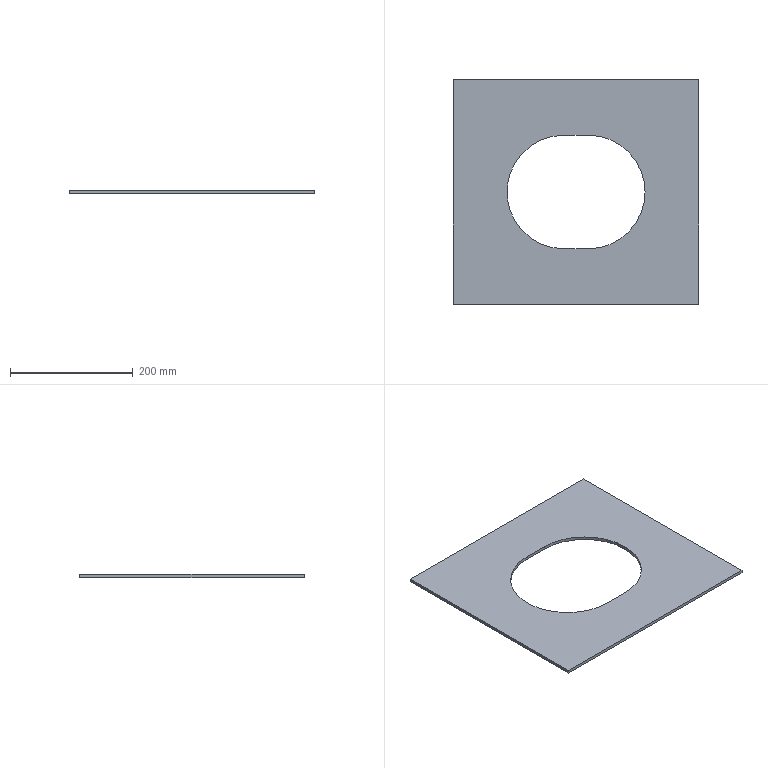Part | SolidWorks | features Extrusion 1, ICE 1 | 1 solid | 11 faces | box 400 x 365 x 5 mm | volume 558599 mm3 | plane 8 | cylinder 3 | commonest cylinder face diameters 185 x3
STEP:
#1=CARTESIAN_POINT('',(312.5,182.5,0.));
#2=VERTEX_POINT('',#1);
#3=CARTESIAN_POINT('',(220.,275.,0.));
#4=VERTEX_POINT('',#3);
#5=CARTESIAN_POINT('',(220.,182.5,0.));
#6=DIRECTION('',(0.,0.,1.));
#7=DIRECTION('',(1.,0.,0.));
#8=AXIS2_PLACEMENT_3D('',#5,#6,#7);
#9=CIRCLE('',#8,92.5);
#10=EDGE_CURVE('',#2,#4,#9,.T.);
#11=ORIENTED_EDGE('',*,*,#10,.F.);
#12=CARTESIAN_POINT('',(312.5,182.5,5.));
#13=VERTEX_POINT('',#12);
#14=CARTESIAN_POINT('',(312.5,182.5,-5.));
#15=DIRECTION('',(0.,0.,1.));
#16=VECTOR('',#15,1000.);
#17=LINE('',#14,#16);
#18=EDGE_CURVE('',#2,#13,#17,.T.);
#19=ORIENTED_EDGE('',*,*,#18,.T.);
#20=CARTESIAN_POINT('',(220.,275.,5.));
#21=VERTEX_POINT('',#20);
#22=CARTESIAN_POINT('',(220.,182.5,5.));
#23=DIRECTION('',(0.,0.,1.));
#24=DIRECTION('',(1.,0.,0.));
#25=AXIS2_PLACEMENT_3D('',#22,#23,#24);
#26=CIRCLE('',#25,92.5);
#27=EDGE_CURVE('',#13,#21,#26,.T.);
#28=ORIENTED_EDGE('',*,*,#27,.T.);
#29=CARTESIAN_POINT('',(220.,275.,-5.));
#30=DIRECTION('',(0.,0.,1.));
#31=VECTOR('',#30,1000.);
#32=LINE('',#29,#31);
#33=EDGE_CURVE('',#4,#21,#32,.T.);
#34=ORIENTED_EDGE('',*,*,#33,.F.);
#35=EDGE_LOOP('',(#11,#19,#28,#34));
#36=FACE_OUTER_BOUND('',#35,.T.);
#37=CARTESIAN_POINT('',(220.,182.5,-5.));
#38=DIRECTION('',(0.,0.,1.));
#39=DIRECTION('',(1.,0.,0.));
#40=AXIS2_PLACEMENT_3D('',#37,#38,#39);
#41=CYLINDRICAL_SURFACE('',#40,92.5);
#42=ADVANCED_FACE('',(#36),#41,.F.);
#43=CARTESIAN_POINT('',(0.,365.,0.));
#44=VERTEX_POINT('',#43);
#45=CARTESIAN_POINT('',(0.,0.,0.));
#46=VERTEX_POINT('',#45);
#47=CARTESIAN_POINT('',(0.,365.,0.));
#48=DIRECTION('',(0.,-1.,0.));
#49=VECTOR('',#48,1000.);
#50=LINE('',#47,#49);
#51=EDGE_CURVE('',#44,#46,#50,.T.);
#52=ORIENTED_EDGE('',*,*,#51,.T.);
#53=CARTESIAN_POINT('',(0.,0.,5.));
#54=VERTEX_POINT('',#53);
#55=CARTESIAN_POINT('',(0.,0.,5.));
#56=DIRECTION('',(0.,0.,-1.));
#57=VECTOR('',#56,1000.);
#58=LINE('',#55,#57);
#59=EDGE_CURVE('',#54,#46,#58,.T.);
#60=ORIENTED_EDGE('',*,*,#59,.F.);
#61=CARTESIAN_POINT('',(0.,365.,5.));
#62=VERTEX_POINT('',#61);
#63=CARTESIAN_POINT('',(0.,365.,5.));
#64=DIRECTION('',(0.,-1.,0.));
#65=VECTOR('',#64,1000.);
#66=LINE('',#63,#65);
#67=EDGE_CURVE('',#62,#54,#66,.T.);
#68=ORIENTED_EDGE('',*,*,#67,.F.);
#69=CARTESIAN_POINT('',(0.,365.,5.));
#70=DIRECTION('',(0.,0.,-1.));
#71=VECTOR('',#70,1000.);
#72=LINE('',#69,#71);
#73=EDGE_CURVE('',#62,#44,#72,.T.);
#74=ORIENTED_EDGE('',*,*,#73,.T.);
#75=EDGE_LOOP('',(#52,#60,#68,#74));
#76=FACE_OUTER_BOUND('',#75,.T.);
#77=CARTESIAN_POINT('',(0.,365.,5.));
#78=DIRECTION('',(1.,0.,0.));
#79=DIRECTION('',(0.,0.,-1.));
#80=AXIS2_PLACEMENT_3D('',#77,#78,#79);
#81=PLANE('',#80);
#82=ADVANCED_FACE('',(#76),#81,.F.);
#83=CARTESIAN_POINT('',(400.,0.,0.));
#84=VERTEX_POINT('',#83);
#85=CARTESIAN_POINT('',(0.,0.,0.));
#86=DIRECTION('',(1.,0.,0.));
#87=VECTOR('',#86,1000.);
#88=LINE('',#85,#87);
#89=EDGE_CURVE('',#46,#84,#88,.T.);
#90=ORIENTED_EDGE('',*,*,#89,.T.);
#91=CARTESIAN_POINT('',(400.,0.,5.));
#92=VERTEX_POINT('',#91);
#93=CARTESIAN_POINT('',(400.,0.,5.));
#94=DIRECTION('',(0.,0.,-1.));
#95=VECTOR('',#94,1000.);
#96=LINE('',#93,#95);
#97=EDGE_CURVE('',#92,#84,#96,.T.);
#98=ORIENTED_EDGE('',*,*,#97,.F.);
#99=CARTESIAN_POINT('',(0.,0.,5.));
#100=DIRECTION('',(1.,0.,0.));
#101=VECTOR('',#100,1000.);
#102=LINE('',#99,#101);
#103=EDGE_CURVE('',#54,#92,#102,.T.);
#104=ORIENTED_EDGE('',*,*,#103,.F.);
#105=ORIENTED_EDGE('',*,*,#59,.T.);
#106=EDGE_LOOP('',(#90,#98,#104,#105));
#107=FACE_OUTER_BOUND('',#106,.T.);
#108=CARTESIAN_POINT('',(0.,0.,5.));
#109=DIRECTION('',(0.,1.,0.));
#110=DIRECTION('',(0.,0.,1.));
#111=AXIS2_PLACEMENT_3D('',#108,#109,#110);
#112=PLANE('',#111);
#113=ADVANCED_FACE('',(#107),#112,.F.);
#114=CARTESIAN_POINT('',(400.,365.,0.));
#115=VERTEX_POINT('',#114);
#116=CARTESIAN_POINT('',(400.,0.,0.));
#117=DIRECTION('',(0.,1.,0.));
#118=VECTOR('',#117,1000.);
#119=LINE('',#116,#118);
#120=EDGE_CURVE('',#84,#115,#119,.T.);
#121=ORIENTED_EDGE('',*,*,#120,.T.);
#122=CARTESIAN_POINT('',(400.,365.,5.));
#123=VERTEX_POINT('',#122);
#124=CARTESIAN_POINT('',(400.,365.,5.));
#125=DIRECTION('',(0.,0.,-1.));
#126=VECTOR('',#125,1000.);
#127=LINE('',#124,#126);
#128=EDGE_CURVE('',#123,#115,#127,.T.);
#129=ORIENTED_EDGE('',*,*,#128,.F.);
#130=CARTESIAN_POINT('',(400.,0.,5.));
#131=DIRECTION('',(0.,1.,0.));
#132=VECTOR('',#131,1000.);
#133=LINE('',#130,#132);
#134=EDGE_CURVE('',#92,#123,#133,.T.);
#135=ORIENTED_EDGE('',*,*,#134,.F.);
#136=ORIENTED_EDGE('',*,*,#97,.T.);
#137=EDGE_LOOP('',(#121,#129,#135,#136));
#138=FACE_OUTER_BOUND('',#137,.T.);
#139=CARTESIAN_POINT('',(400.,0.,5.));
#140=DIRECTION('',(-1.,0.,0.));
#141=DIRECTION('',(0.,0.,1.));
#142=AXIS2_PLACEMENT_3D('',#139,#140,#141);
#143=PLANE('',#142);
#144=ADVANCED_FACE('',(#138),#143,.F.);
#145=CARTESIAN_POINT('',(400.,365.,0.));
#146=DIRECTION('',(-1.,0.,0.));
#147=VECTOR('',#146,1000.);
#148=LINE('',#145,#147);
#149=EDGE_CURVE('',#115,#44,#148,.T.);
#150=ORIENTED_EDGE('',*,*,#149,.T.);
#151=ORIENTED_EDGE('',*,*,#73,.F.);
#152=CARTESIAN_POINT('',(400.,365.,5.));
#153=DIRECTION('',(-1.,0.,0.));
#154=VECTOR('',#153,1000.);
#155=LINE('',#152,#154);
#156=EDGE_CURVE('',#123,#62,#155,.T.);
#157=ORIENTED_EDGE('',*,*,#156,.F.);
#158=ORIENTED_EDGE('',*,*,#128,.T.);
#159=EDGE_LOOP('',(#150,#151,#157,#158));
#160=FACE_OUTER_BOUND('',#159,.T.);
#161=CARTESIAN_POINT('',(400.,365.,5.));
#162=DIRECTION('',(0.,-1.,0.));
#163=DIRECTION('',(0.,0.,-1.));
#164=AXIS2_PLACEMENT_3D('',#161,#162,#163);
#165=PLANE('',#164);
#166=ADVANCED_FACE('',(#160),#165,.F.);
#167=CARTESIAN_POINT('',(180.,275.,5.));
#168=VERTEX_POINT('',#167);
#169=CARTESIAN_POINT('',(180.,90.,5.));
#170=VERTEX_POINT('',#169);
#171=CARTESIAN_POINT('',(180.,182.5,5.));
#172=DIRECTION('',(0.,0.,1.));
#173=DIRECTION('',(1.,0.,0.));
#174=AXIS2_PLACEMENT_3D('',#171,#172,#173);
#175=CIRCLE('',#174,92.5);
#176=EDGE_CURVE('',#168,#170,#175,.T.);
#177=ORIENTED_EDGE('',*,*,#176,.F.);
#178=CARTESIAN_POINT('',(180.,275.,5.));
#179=DIRECTION('',(-1.,0.,0.));
#180=VECTOR('',#179,1000.);
#181=LINE('',#178,#180);
#182=EDGE_CURVE('',#21,#168,#181,.T.);
#183=ORIENTED_EDGE('',*,*,#182,.F.);
#184=ORIENTED_EDGE('',*,*,#27,.F.);
#185=CARTESIAN_POINT('',(220.,90.,5.));
#186=VERTEX_POINT('',#185);
#187=CARTESIAN_POINT('',(220.,182.5,5.));
#188=DIRECTION('',(0.,0.,1.));
#189=DIRECTION('',(1.,0.,0.));
#190=AXIS2_PLACEMENT_3D('',#187,#188,#189);
#191=CIRCLE('',#190,92.5);
#192=EDGE_CURVE('',#186,#13,#191,.T.);
#193=ORIENTED_EDGE('',*,*,#192,.F.);
#194=CARTESIAN_POINT('',(180.,90.,5.));
#195=DIRECTION('',(1.,0.,0.));
#196=VECTOR('',#195,1000.);
#197=LINE('',#194,#196);
#198=EDGE_CURVE('',#170,#186,#197,.T.);
#199=ORIENTED_EDGE('',*,*,#198,.F.);
#200=EDGE_LOOP('',(#177,#183,#184,#193,#199));
#201=FACE_BOUND('',#200,.T.);
#202=ORIENTED_EDGE('',*,*,#67,.T.);
#203=ORIENTED_EDGE('',*,*,#103,.T.);
#204=ORIENTED_EDGE('',*,*,#134,.T.);
#205=ORIENTED_EDGE('',*,*,#156,.T.);
#206=EDGE_LOOP('',(#202,#203,#204,#205));
#207=FACE_OUTER_BOUND('',#206,.T.);
#208=CARTESIAN_POINT('',(0.,0.,5.));
#209=DIRECTION('',(0.,0.,1.));
#210=DIRECTION('',(1.,0.,0.));
#211=AXIS2_PLACEMENT_3D('',#208,#209,#210);
#212=PLANE('',#211);
#213=ADVANCED_FACE('',(#201,#207),#212,.T.);
#214=CARTESIAN_POINT('',(180.,275.,0.));
#215=VERTEX_POINT('',#214);
#216=CARTESIAN_POINT('',(0.,275.,0.));
#217=DIRECTION('',(-1.,0.,0.));
#218=VECTOR('',#217,1000.);
#219=LINE('',#216,#218);
#220=EDGE_CURVE('',#4,#215,#219,.T.);
#221=ORIENTED_EDGE('',*,*,#220,.T.);
#222=CARTESIAN_POINT('',(180.,90.,0.));
#223=VERTEX_POINT('',#222);
#224=CARTESIAN_POINT('',(180.,182.5,0.));
#225=DIRECTION('',(0.,0.,1.));
#226=DIRECTION('',(1.,0.,0.));
#227=AXIS2_PLACEMENT_3D('',#224,#225,#226);
#228=CIRCLE('',#227,92.5);
#229=EDGE_CURVE('',#215,#223,#228,.T.);
#230=ORIENTED_EDGE('',*,*,#229,.T.);
#231=CARTESIAN_POINT('',(220.,90.,0.));
#232=VERTEX_POINT('',#231);
#233=CARTESIAN_POINT('',(0.,90.,0.));
#234=DIRECTION('',(1.,0.,0.));
#235=VECTOR('',#234,1000.);
#236=LINE('',#233,#235);
#237=EDGE_CURVE('',#223,#232,#236,.T.);
#238=ORIENTED_EDGE('',*,*,#237,.T.);
#239=CARTESIAN_POINT('',(220.,182.5,0.));
#240=DIRECTION('',(0.,0.,1.));
#241=DIRECTION('',(1.,0.,0.));
#242=AXIS2_PLACEMENT_3D('',#239,#240,#241);
#243=CIRCLE('',#242,92.5);
#244=EDGE_CURVE('',#232,#2,#243,.T.);
#245=ORIENTED_EDGE('',*,*,#244,.T.);
#246=ORIENTED_EDGE('',*,*,#10,.T.);
#247=EDGE_LOOP('',(#221,#230,#238,#245,#246));
#248=FACE_BOUND('',#247,.T.);
#249=ORIENTED_EDGE('',*,*,#51,.F.);
#250=ORIENTED_EDGE('',*,*,#149,.F.);
#251=ORIENTED_EDGE('',*,*,#120,.F.);
#252=ORIENTED_EDGE('',*,*,#89,.F.);
#253=EDGE_LOOP('',(#249,#250,#251,#252));
#254=FACE_OUTER_BOUND('',#253,.T.);
#255=CARTESIAN_POINT('',(0.,0.,0.));
#256=DIRECTION('',(0.,0.,1.));
#257=DIRECTION('',(1.,0.,0.));
#258=AXIS2_PLACEMENT_3D('',#255,#256,#257);
#259=PLANE('',#258);
#260=ADVANCED_FACE('',(#248,#254),#259,.F.);
#261=CARTESIAN_POINT('',(180.,275.,-5.));
#262=DIRECTION('',(0.,0.,1.));
#263=VECTOR('',#262,1000.);
#264=LINE('',#261,#263);
#265=EDGE_CURVE('',#215,#168,#264,.T.);
#266=ORIENTED_EDGE('',*,*,#265,.T.);
#267=ORIENTED_EDGE('',*,*,#176,.T.);
#268=CARTESIAN_POINT('',(180.,90.,-5.));
#269=DIRECTION('',(0.,0.,1.));
#270=VECTOR('',#269,1000.);
#271=LINE('',#268,#270);
#272=EDGE_CURVE('',#223,#170,#271,.T.);
#273=ORIENTED_EDGE('',*,*,#272,.F.);
#274=ORIENTED_EDGE('',*,*,#229,.F.);
#275=EDGE_LOOP('',(#266,#267,#273,#274));
#276=FACE_OUTER_BOUND('',#275,.T.);
#277=CARTESIAN_POINT('',(180.,182.5,-5.));
#278=DIRECTION('',(0.,0.,1.));
#279=DIRECTION('',(1.,0.,0.));
#280=AXIS2_PLACEMENT_3D('',#277,#278,#279);
#281=CYLINDRICAL_SURFACE('',#280,92.5);
#282=ADVANCED_FACE('',(#276),#281,.F.);
#283=ORIENTED_EDGE('',*,*,#33,.T.);
#284=ORIENTED_EDGE('',*,*,#182,.T.);
#285=ORIENTED_EDGE('',*,*,#265,.F.);
#286=ORIENTED_EDGE('',*,*,#220,.F.);
#287=EDGE_LOOP('',(#283,#284,#285,#286));
#288=FACE_OUTER_BOUND('',#287,.T.);
#289=CARTESIAN_POINT('',(180.,275.,-5.));
#290=DIRECTION('',(0.,1.,0.));
#291=DIRECTION('',(0.,0.,1.));
#292=AXIS2_PLACEMENT_3D('',#289,#290,#291);
#293=PLANE('',#292);
#294=ADVANCED_FACE('',(#288),#293,.F.);
#295=ORIENTED_EDGE('',*,*,#18,.F.);
#296=ORIENTED_EDGE('',*,*,#244,.F.);
#297=CARTESIAN_POINT('',(220.,90.,-5.));
#298=DIRECTION('',(0.,0.,1.));
#299=VECTOR('',#298,1000.);
#300=LINE('',#297,#299);
#301=EDGE_CURVE('',#232,#186,#300,.T.);
#302=ORIENTED_EDGE('',*,*,#301,.T.);
#303=ORIENTED_EDGE('',*,*,#192,.T.);
#304=EDGE_LOOP('',(#295,#296,#302,#303));
#305=FACE_OUTER_BOUND('',#304,.T.);
#306=CARTESIAN_POINT('',(220.,182.5,-5.));
#307=DIRECTION('',(0.,0.,1.));
#308=DIRECTION('',(1.,0.,0.));
#309=AXIS2_PLACEMENT_3D('',#306,#307,#308);
#310=CYLINDRICAL_SURFACE('',#309,92.5);
#311=ADVANCED_FACE('',(#305),#310,.F.);
#312=ORIENTED_EDGE('',*,*,#272,.T.);
#313=ORIENTED_EDGE('',*,*,#198,.T.);
#314=ORIENTED_EDGE('',*,*,#301,.F.);
#315=ORIENTED_EDGE('',*,*,#237,.F.);
#316=EDGE_LOOP('',(#312,#313,#314,#315));
#317=FACE_OUTER_BOUND('',#316,.T.);
#318=CARTESIAN_POINT('',(180.,90.,-5.));
#319=DIRECTION('',(0.,-1.,0.));
#320=DIRECTION('',(0.,0.,-1.));
#321=AXIS2_PLACEMENT_3D('',#318,#319,#320);
#322=PLANE('',#321);
#323=ADVANCED_FACE('',(#317),#322,.F.);
#324=CLOSED_SHELL('',(#42,#82,#113,#144,#166,#213,#260,#282,#294,#311,#323));
#325=MANIFOLD_SOLID_BREP('',#324);
#326=CARTESIAN_POINT('',(0.,0.,0.));
#327=DIRECTION('',(0.,0.,1.));
#328=DIRECTION('',(1.,0.,0.));
#329=AXIS2_PLACEMENT_3D('',#326,#327,#328);
#330=(LENGTH_UNIT()NAMED_UNIT(*)SI_UNIT(.MILLI.,.METRE.));
#331=UNCERTAINTY_MEASURE_WITH_UNIT(LENGTH_MEASURE(0.00001),#330,'','');
#332=(NAMED_UNIT(*)PLANE_ANGLE_UNIT()SI_UNIT($,.RADIAN.));
#333=(NAMED_UNIT(*)SI_UNIT($,.STERADIAN.)SOLID_ANGLE_UNIT());
#334=(GEOMETRIC_REPRESENTATION_CONTEXT(3)GLOBAL_UNCERTAINTY_ASSIGNED_CONTEXT((#331))GLOBAL_UNIT_ASSIGNED_CONTEXT((#330,#332,#333))REPRESENTATION_CONTEXT('',''));
#335=ADVANCED_BREP_SHAPE_REPRESENTATION('',(#325,#329),#334);